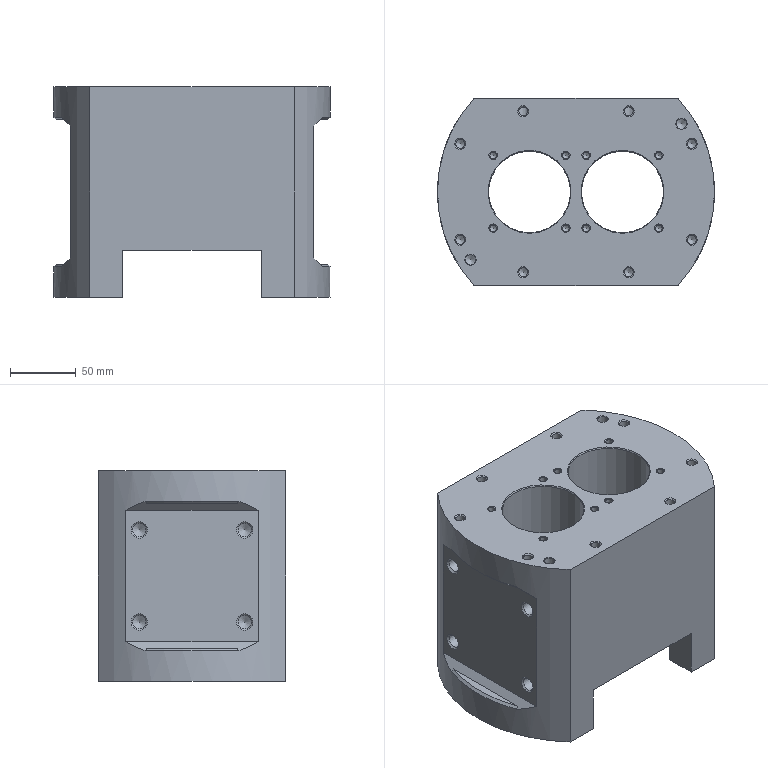NC program | NX | posted with a generic post | part box 210 x 142 x 160 mm
Lines 1 to 469 of 4789:
N10 G17 G21 G94 G90
(FLOOR_WALL_COPY_1_COPY , TOOL : D50)
N12 T02 M6
N14 G54
N16 G17 G0 G90 X-25.097 Y-36.47 B0. C0. S1200 M3
N18 G43 Z30. H2
N20 Z2.658
N22 G94 G1 Z-0.342 F1000.
N24 Y-33.47
N26 Y33.47 F2000.
N28 X0.001
N30 Y-33.47
N32 X25.1
N34 Y33.47
N36 Y36.47
N38 Z2.658
N40 G0 Z30.
N42 X-25.097 Y-39.966
N44 Z2.316
N46 G1 Z-0.684 F1000.
N48 Y-36.966
N50 Y36.966 F2000.
N52 X0.001
N54 Y-36.966
N56 X25.1
N58 Y36.966
N60 Y39.966
N62 Z2.316
N64 G0 Z30.
N66 X-25.097 Y-42.642
N68 Z1.974
N70 G1 Z-1.026 F1000.
N72 Y-39.642
N74 Y39.642 F2000.
N76 X0.001
N78 Y-39.642
N80 X25.1
N82 Y39.642
N84 Y42.642
N86 Z1.974
N88 G0 Z30.
N90 X-25.097 Y-44.893
N92 Z1.632
N94 G1 Z-1.368 F1000.
N96 Y-41.893
N98 Y41.893 F2000.
N100 X0.001
N102 Y-41.893
N104 X25.1
N106 Y41.893
N108 Y44.893
N110 Z1.632
N112 G0 Z30.
N114 X-25.097 Y-46.871
N116 Z1.29
N118 G1 Z-1.71 F1000.
N120 Y-43.871
N122 Y43.871 F2000.
N124 X0.001
N126 Y-43.871
N128 X25.1
N130 Y43.871
N132 Y46.871
N134 Z1.29
N136 G0 Z30.
N138 X-25.097 Y-48.655
N140 Z0.948
N142 G1 Z-2.052 F1000.
N144 Y-45.655
N146 Y45.655 F2000.
N148 X0.001
N150 Y-45.655
N152 X25.1
N154 Y45.655
N156 Y48.655
N158 Z0.948
N160 G0 Z30.
N162 X-25.097 Y-50.291
N164 Z0.607
N166 G1 Z-2.393 F1000.
N168 Y-47.291
N170 Y47.291 F2000.
N172 X0.001
N174 Y-47.291
N176 X25.1
N178 Y47.291
N180 Y50.291
N182 Z0.607
N184 G0 Z30.
N186 X-25.097 Y-51.811
N188 Z0.265
N190 G1 Z-2.735 F1000.
N192 Y-48.811
N194 Y48.811 F2000.
N196 X0.001
N198 Y-48.811
N200 X25.1
N202 Y48.811
N204 Y51.811
N206 Z0.265
N208 G0 Z30.
N210 X-25.097 Y-53.234
N212 Z-0.077
N214 G1 Z-3.077 F1000.
N216 Y-50.234
N218 Y50.234 F2000.
N220 X0.001
N222 Y-50.234
N224 X25.1
N226 Y50.234
N228 Y53.234
N230 Z-0.077
N232 G0 Z30.
N234 X-25.097 Y-54.577
N236 Z-0.419
N238 G1 Z-3.419 F1000.
N240 Y-51.577
N242 Y51.577 F2000.
N244 X0.001
N246 Y-51.577
N248 X25.1
N250 Y51.577
N252 Y54.577
N254 Z-0.419
N256 G0 Z30.
N258 X-25.097 Y-55.851
N260 Z-0.761
N262 G1 Z-3.761 F1000.
N264 Y-52.851
N266 Y52.851 F2000.
N268 X0.001
N270 Y-52.851
N272 X25.1
N274 Y52.851
N276 Y55.851
N278 Z-0.761
N280 G0 Z30.
N282 X-25.097 Y-57.065
N284 Z-1.103
N286 G1 Z-4.103 F1000.
N288 Y-54.065
N290 Y54.065 F2000.
N292 X0.001
N294 Y-54.065
N296 X25.1
N298 Y54.065
N300 Y57.065
N302 Z-1.103
N304 G0 Z30.
N306 X-25.097 Y-58.227
N308 Z-1.445
N310 G1 Z-4.445 F1000.
N312 Y-55.227
N314 Y55.227 F2000.
N316 X0.001
N318 Y-55.227
N320 X25.1
N322 Y55.227
N324 Y58.227
N326 Z-1.445
N328 G0 Z30.
N330 X-25.097 Y-59.341
N332 Z-1.787
N334 G1 Z-4.787 F1000.
N336 Y-56.341
N338 Y56.341 F2000.
N340 X0.001
N342 Y-56.341
N344 X25.1
N346 Y56.341
N348 Y59.341
N350 Z-1.787
N352 G0 Z30.
N354 X-25.097 Y-60.414
N356 Z-2.129
N358 G1 Z-5.129 F1000.
N360 Y-57.414
N362 Y57.414 F2000.
N364 X0.001
N366 Y-57.414
N368 X25.1
N370 Y57.414
N372 Y60.414
N374 Z-2.129
N376 G0 Z30.
N378 X-25.097 Y-61.449
N380 Z-2.47
N382 G1 Z-5.47 F1000.
N384 Y-58.449
N386 Y58.449 F2000.
N388 X0.001
N390 Y-58.449
N392 X25.1
N394 Y58.449
N396 Y61.449
N398 Z-2.47
N400 G0 Z30.
N402 X-25.097 Y-62.45
N404 Z-2.812
N406 G1 Z-5.812 F1000.
N408 Y-59.45
N410 Y59.45 F2000.
N412 X0.001
N414 Y-59.45
N416 X25.1
N418 Y59.45
N420 Y62.45
N422 Z-2.812
N424 G0 Z30.
N426 X-25.097 Y-63.419
N428 Z-3.154
N430 G1 Z-6.154 F1000.
N432 Y-60.419
N434 Y60.419 F2000.
N436 X0.001
N438 Y-60.419
N440 X25.1
N442 Y60.419
N444 Y63.419
N446 Z-3.154
N448 G0 Z30.
N450 X-25.097 Y-64.359
N452 Z-3.496
N454 G1 Z-6.496 F1000.
N456 Y-61.359
N458 Y61.359 F2000.
N460 X0.001
N462 Y-61.359
N464 X25.1
N466 Y61.359
N468 Y64.359
N470 Z-3.496
N472 G0 Z30.
N474 X-25.097 Y-65.272
N476 Z-3.838
N478 G1 Z-6.838 F1000.
N480 Y-62.272
N482 Y62.272 F2000.
N484 X0.001
N486 Y-62.272
N488 X25.1
N490 Y62.272
N492 Y65.272
N494 Z-3.838
N496 G0 Z30.
N498 X-25.097 Y-66.16
N500 Z-4.18
N502 G1 Z-7.18 F1000.
N504 Y-63.16
N506 Y63.16 F2000.
N508 X0.001
N510 Y-63.16
N512 X25.1
N514 Y63.16
N516 Y66.16
N518 Z-4.18
N520 G0 Z30.
N522 X-25.097 Y-67.025
N524 Z-4.522
N526 G1 Z-7.522 F1000.
N528 Y-64.025
N530 Y64.025 F2000.
N532 X0.001
N534 Y-64.025
N536 X25.1
N538 Y64.025
N540 Y67.025
N542 Z-4.522
N544 G0 Z30.
N546 X-25.097 Y-67.869
N548 Z-4.864
N550 G1 Z-7.864 F1000.
N552 Y-64.869
N554 Y64.869 F2000.
N556 X0.001
N558 Y-64.869
N560 X25.1
N562 Y64.869
N564 Y67.869
N566 Z-4.864
N568 G0 Z30.
N570 X-25.097 Y-68.692
N572 Z-5.206
N574 G1 Z-8.206 F1000.
N576 Y-65.692
N578 Y65.692 F2000.
N580 X0.001
N582 Y-65.692
N584 X25.1
N586 Y65.692
N588 Y68.692
N590 Z-5.206
N592 G0 Z30.
N594 X-25.097 Y-69.496
N596 Z-5.547
N598 G1 Z-8.547 F1000.
N600 Y-66.496
N602 Y66.496 F2000.
N604 X0.001
N606 Y-66.496
N608 X25.1
N610 Y66.496
N612 Y69.496
N614 Z-5.547
N616 G0 Z30.
N618 X-25.097 Y-70.282
N620 Z-5.889
N622 G1 Z-8.889 F1000.
N624 Y-67.282
N626 Y67.282 F2000.
N628 X0.001
N630 Y-67.282
N632 X25.1
N634 Y67.282
N636 Y70.282
N638 Z-5.889
N640 G0 Z30.
N642 X-25.097 Y-71.05
N644 Z-6.231
N646 G1 Z-9.231 F1000.
N648 Y-68.05
N650 Y68.05 F2000.
N652 X0.001
N654 Y-68.05
N656 X25.1
N658 Y68.05
N660 Y71.05
N662 Z-6.231
N664 G0 Z30.
N666 X-25.097 Y-71.803
N668 Z-6.573
N670 G1 Z-9.573 F1000.
N672 Y-68.803
N674 Y68.803 F2000.
N676 X0.001
N678 Y-68.803
N680 X25.1
N682 Y68.803
N684 Y71.803
N686 Z-6.573
N688 G0 Z30.
N690 X-25.097 Y-72.54
N692 Z-6.915
N694 G1 Z-9.915 F1000.
N696 Y-69.54
N698 Y69.54 F2000.
N700 X0.001
N702 Y-69.54
N704 X25.1
N706 Y69.54
N708 Y72.54
N710 Z-6.915
N712 G0 Z30.
N714 X-25.097 Y-73.263
N716 Z-7.257
N718 G1 Z-10.257 F1000.
N720 Y-70.263
N722 Y70.263 F2000.
N724 X0.001
N726 Y-70.263
N728 X25.1
N730 Y70.263
N732 Y73.263
N734 Z-7.257
N736 G0 Z30.
N738 X-25.097 Y-73.972
N740 Z-7.599
N742 G1 Z-10.599 F1000.
N744 Y-70.972
N746 Y70.972 F2000.
N748 X0.001
N750 Y-70.972
N752 X25.1
N754 Y70.972
N756 Y73.972
N758 Z-7.599
N760 G0 Z30.
N762 X-25.097 Y-74.667
N764 Z-7.941
N766 G1 Z-10.941 F1000.
N768 Y-71.667
N770 Y71.667 F2000.
N772 X0.001
N774 Y-71.667
N776 X25.1
N778 Y71.667
N780 Y74.667
N782 Z-7.941
N784 G0 Z30.
N786 X-25.097 Y-75.35
N788 Z-8.282
N790 G1 Z-11.282 F1000.
N792 Y-72.35
N794 Y72.35 F2000.
N796 X0.001
N798 Y-72.35
N800 X25.1
N802 Y72.35
N804 Y75.35
N806 Z-8.282
N808 G0 Z30.
N810 X-25.097 Y-76.021
N812 Z-8.624
N814 G1 Z-11.624 F1000.
N816 Y-73.021
N818 Y73.021 F2000.
N820 X0.001
N822 Y-73.021
N824 X25.1
N826 Y73.021
N828 Y76.021
N830 Z-8.624
N832 G0 Z30.
N834 X-25.097 Y-76.68
N836 Z-8.966
N838 G1 Z-11.966 F1000.
N840 Y-73.68
N842 Y73.68 F2000.
N844 X0.001
N846 Y-73.68
N848 X25.1
N850 Y73.68
N852 Y76.68
N854 Z-8.966
N856 G0 Z30.
N858 X-25.097 Y-77.328
N860 Z-9.308
N862 G1 Z-12.308 F1000.
N864 Y-74.328
N866 Y74.328 F2000.
N868 X0.001
N870 Y-74.328
N872 X25.1
N874 Y74.328
N876 Y77.328
N878 Z-9.308
N880 G0 Z30.
N882 X-25.097 Y-77.965
N884 Z-9.65
N886 G1 Z-12.65 F1000.
N888 Y-74.965
N890 Y74.965 F2000.
N892 X0.001
N894 Y-74.965
N896 X25.1
N898 Y74.965
N900 Y77.965
N902 Z-9.65
N904 G0 Z30.
(FLOOR_WALL_COPY_COPY_COPY , TOOL : D50)
N906 X-24.997 Y-78.149 S2500
N908 Z-9.75
N910 G1 Z-12.75 F1000.
N912 Y-75.149
N914 Y75.149
N916 X0.001
N918 Y-75.149
N920 X25.
N922 Y75.149
N924 Y78.149
N926 Z-9.75
N928 G0 Z30.
N930 M5